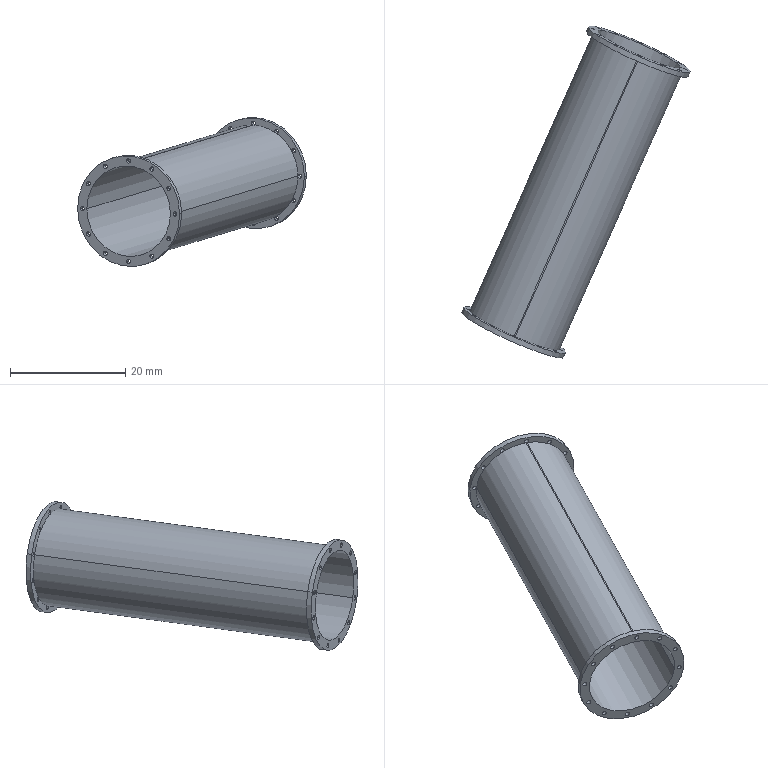Part | SolidWorks | features SplitBody 1 | 1 solid | 82 faces | box 39.711 x 57.638 x 25.888 mm | volume 1596 mm3 | cylinder 56 | plane 26 | commonest cylinder face diameters 0.739 x47 19.36 x4 16.896 x3 15.84 x2